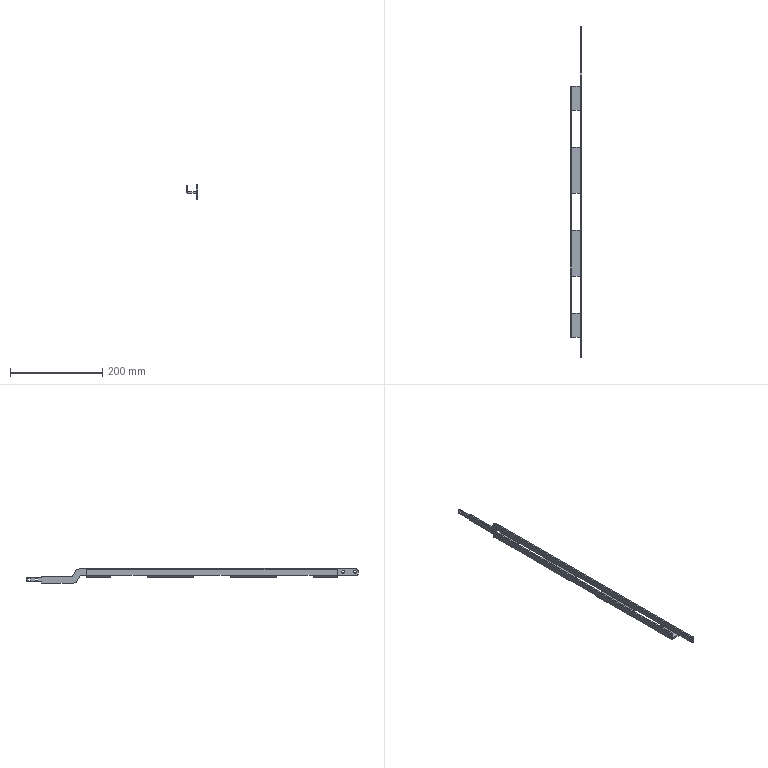Part | SolidWorks | features BaseBody 1 | 1 solid | 85 faces | box 25 x 721 x 30.5 mm | volume 74110 mm3 | plane 57 | cylinder 28 | commonest cylinder face diameters 6 x10 1 x8 7 x8 20 x2